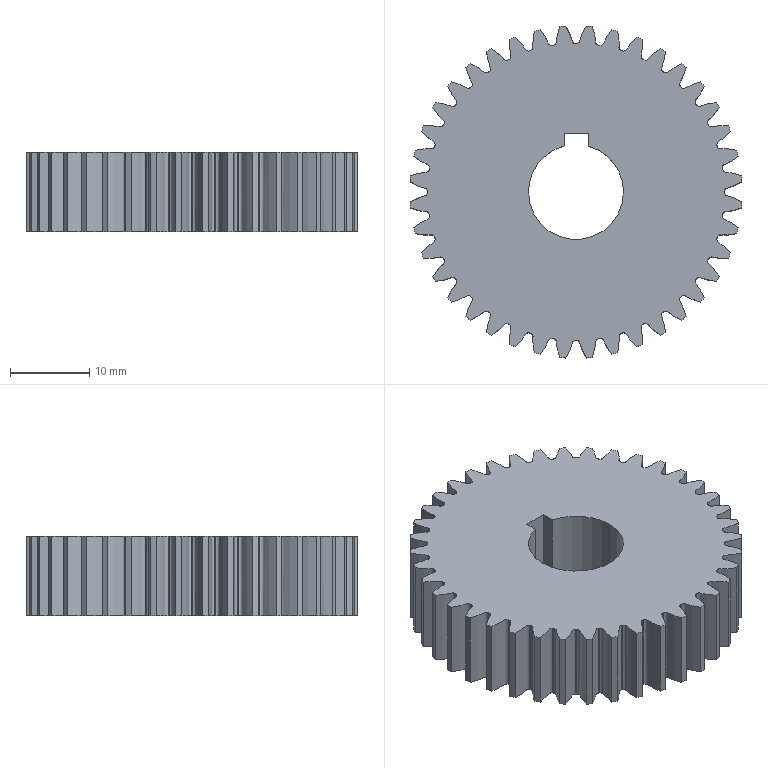Part | SolidWorks | features ICE 3, CirPattern 1, Extrusion 1, RefAxis 1 | 1 solid | 171 faces | box 41.923 x 41.923 x 10 mm | volume 11284 mm3 | cylinder 86 | spline 80 | plane 5 | commonest cylinder face diameters 37.5 x41 42 x40 12 x3 3 x2